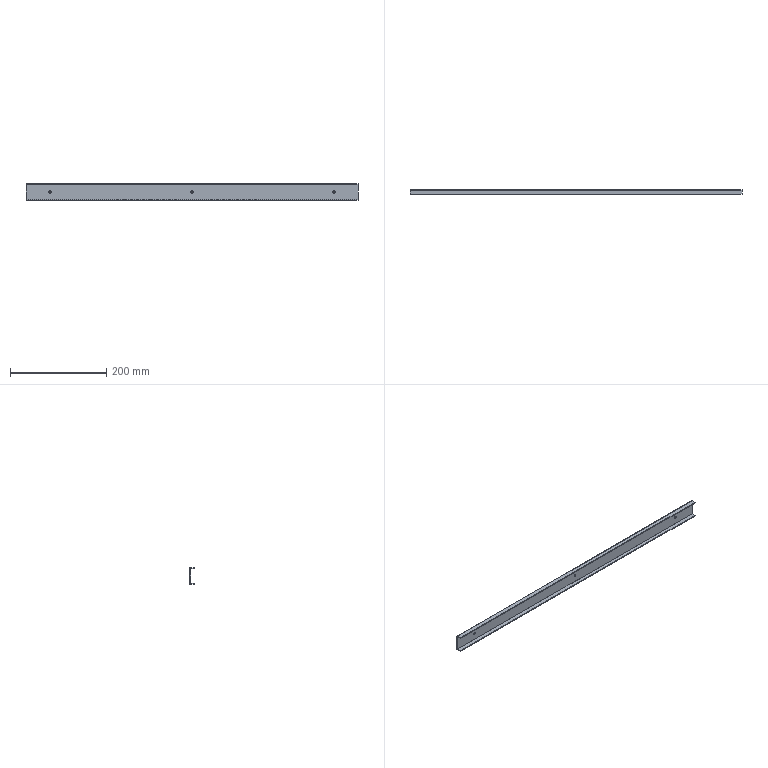Part | STEP file | Sliding Door Spacer Block | 1 solid | 20 faces | box 690 x 10 x 35 mm | volume 68950 mm3 | cylinder 10 | plane 10 | commonest cylinder face diameters 5.2 x6 0.2 x2 4.2 x2
STEP:
#1=CARTESIAN_POINT('',(-30.031,-2.,2.333));
#2=VERTEX_POINT('',#1);
#3=CARTESIAN_POINT('',(-30.031,-2.,-2.867));
#4=VERTEX_POINT('',#3);
#5=CARTESIAN_POINT('',(-30.031,-2.,-0.2666));
#6=DIRECTION('',(0.,-1.,0.));
#7=DIRECTION('',(0.,0.,1.));
#8=AXIS2_PLACEMENT_3D('',#5,#6,#7);
#9=CIRCLE('',#8,2.6);
#10=EDGE_CURVE('',#2,#4,#9,.T.);
#11=ORIENTED_EDGE('',*,*,#10,.T.);
#12=CARTESIAN_POINT('',(-30.031,0.,-2.867));
#13=VERTEX_POINT('',#12);
#14=CARTESIAN_POINT('',(-30.031,-2.,-2.867));
#15=DIRECTION('',(0.,1.,0.));
#16=VECTOR('',#15,1000.);
#17=LINE('',#14,#16);
#18=EDGE_CURVE('',#4,#13,#17,.T.);
#19=ORIENTED_EDGE('',*,*,#18,.T.);
#20=CARTESIAN_POINT('',(-30.031,0.,2.333));
#21=VERTEX_POINT('',#20);
#22=CARTESIAN_POINT('',(-30.031,0.,-0.2666));
#23=DIRECTION('',(0.,-1.,0.));
#24=DIRECTION('',(0.,0.,1.));
#25=AXIS2_PLACEMENT_3D('',#22,#23,#24);
#26=CIRCLE('',#25,2.6);
#27=EDGE_CURVE('',#21,#13,#26,.T.);
#28=ORIENTED_EDGE('',*,*,#27,.F.);
#29=CARTESIAN_POINT('',(-30.031,-2.,2.333));
#30=DIRECTION('',(0.,1.,0.));
#31=VECTOR('',#30,1000.);
#32=LINE('',#29,#31);
#33=EDGE_CURVE('',#2,#21,#32,.T.);
#34=ORIENTED_EDGE('',*,*,#33,.F.);
#35=EDGE_LOOP('',(#11,#19,#28,#34));
#36=FACE_OUTER_BOUND('',#35,.T.);
#37=CARTESIAN_POINT('',(-30.031,-2.,-0.2666));
#38=DIRECTION('',(0.,1.,0.));
#39=DIRECTION('',(0.,0.,1.));
#40=AXIS2_PLACEMENT_3D('',#37,#38,#39);
#41=CYLINDRICAL_SURFACE('',#40,2.6);
#42=ADVANCED_FACE('',(#36),#41,.F.);
#43=CARTESIAN_POINT('',(264.969,-2.,2.333));
#44=VERTEX_POINT('',#43);
#45=CARTESIAN_POINT('',(264.969,-2.,-2.867));
#46=VERTEX_POINT('',#45);
#47=CARTESIAN_POINT('',(264.969,-2.,-0.2666));
#48=DIRECTION('',(0.,-1.,0.));
#49=DIRECTION('',(0.,0.,1.));
#50=AXIS2_PLACEMENT_3D('',#47,#48,#49);
#51=CIRCLE('',#50,2.6);
#52=EDGE_CURVE('',#44,#46,#51,.T.);
#53=ORIENTED_EDGE('',*,*,#52,.T.);
#54=CARTESIAN_POINT('',(264.969,0.,-2.867));
#55=VERTEX_POINT('',#54);
#56=CARTESIAN_POINT('',(264.969,-2.,-2.867));
#57=DIRECTION('',(0.,1.,0.));
#58=VECTOR('',#57,1000.);
#59=LINE('',#56,#58);
#60=EDGE_CURVE('',#46,#55,#59,.T.);
#61=ORIENTED_EDGE('',*,*,#60,.T.);
#62=CARTESIAN_POINT('',(264.969,0.,2.333));
#63=VERTEX_POINT('',#62);
#64=CARTESIAN_POINT('',(264.969,0.,-0.2666));
#65=DIRECTION('',(0.,-1.,0.));
#66=DIRECTION('',(0.,0.,1.));
#67=AXIS2_PLACEMENT_3D('',#64,#65,#66);
#68=CIRCLE('',#67,2.6);
#69=EDGE_CURVE('',#63,#55,#68,.T.);
#70=ORIENTED_EDGE('',*,*,#69,.F.);
#71=CARTESIAN_POINT('',(264.969,-2.,2.333));
#72=DIRECTION('',(0.,1.,0.));
#73=VECTOR('',#72,1000.);
#74=LINE('',#71,#73);
#75=EDGE_CURVE('',#44,#63,#74,.T.);
#76=ORIENTED_EDGE('',*,*,#75,.F.);
#77=EDGE_LOOP('',(#53,#61,#70,#76));
#78=FACE_OUTER_BOUND('',#77,.T.);
#79=CARTESIAN_POINT('',(264.969,-2.,-0.2666));
#80=DIRECTION('',(0.,1.,0.));
#81=DIRECTION('',(0.,0.,1.));
#82=AXIS2_PLACEMENT_3D('',#79,#80,#81);
#83=CYLINDRICAL_SURFACE('',#82,2.6);
#84=ADVANCED_FACE('',(#78),#83,.F.);
#85=CARTESIAN_POINT('',(559.969,-2.,2.333));
#86=VERTEX_POINT('',#85);
#87=CARTESIAN_POINT('',(559.969,-2.,-2.867));
#88=VERTEX_POINT('',#87);
#89=CARTESIAN_POINT('',(559.969,-2.,-0.2666));
#90=DIRECTION('',(0.,-1.,0.));
#91=DIRECTION('',(0.,0.,1.));
#92=AXIS2_PLACEMENT_3D('',#89,#90,#91);
#93=CIRCLE('',#92,2.6);
#94=EDGE_CURVE('',#86,#88,#93,.T.);
#95=ORIENTED_EDGE('',*,*,#94,.T.);
#96=CARTESIAN_POINT('',(559.969,0.,-2.867));
#97=VERTEX_POINT('',#96);
#98=CARTESIAN_POINT('',(559.969,-2.,-2.867));
#99=DIRECTION('',(0.,1.,0.));
#100=VECTOR('',#99,1000.);
#101=LINE('',#98,#100);
#102=EDGE_CURVE('',#88,#97,#101,.T.);
#103=ORIENTED_EDGE('',*,*,#102,.T.);
#104=CARTESIAN_POINT('',(559.969,0.,2.333));
#105=VERTEX_POINT('',#104);
#106=CARTESIAN_POINT('',(559.969,0.,-0.2666));
#107=DIRECTION('',(0.,-1.,0.));
#108=DIRECTION('',(0.,0.,1.));
#109=AXIS2_PLACEMENT_3D('',#106,#107,#108);
#110=CIRCLE('',#109,2.6);
#111=EDGE_CURVE('',#105,#97,#110,.T.);
#112=ORIENTED_EDGE('',*,*,#111,.F.);
#113=CARTESIAN_POINT('',(559.969,-2.,2.333));
#114=DIRECTION('',(0.,1.,0.));
#115=VECTOR('',#114,1000.);
#116=LINE('',#113,#115);
#117=EDGE_CURVE('',#86,#105,#116,.T.);
#118=ORIENTED_EDGE('',*,*,#117,.F.);
#119=EDGE_LOOP('',(#95,#103,#112,#118));
#120=FACE_OUTER_BOUND('',#119,.T.);
#121=CARTESIAN_POINT('',(559.969,-2.,-0.2666));
#122=DIRECTION('',(0.,1.,0.));
#123=DIRECTION('',(0.,0.,1.));
#124=AXIS2_PLACEMENT_3D('',#121,#122,#123);
#125=CYLINDRICAL_SURFACE('',#124,2.6);
#126=ADVANCED_FACE('',(#120),#125,.F.);
#127=CARTESIAN_POINT('',(609.969,-2.,15.133));
#128=VERTEX_POINT('',#127);
#129=CARTESIAN_POINT('',(609.969,-2.,-15.667));
#130=VERTEX_POINT('',#129);
#131=CARTESIAN_POINT('',(609.969,-2.,0.));
#132=DIRECTION('',(0.,0.,-1.));
#133=VECTOR('',#132,1000.);
#134=LINE('',#131,#133);
#135=EDGE_CURVE('',#128,#130,#134,.T.);
#136=ORIENTED_EDGE('',*,*,#135,.F.);
#137=CARTESIAN_POINT('',(-80.031,-2.,15.133));
#138=VERTEX_POINT('',#137);
#139=CARTESIAN_POINT('',(0.,-2.,15.133));
#140=DIRECTION('',(1.,0.,0.));
#141=VECTOR('',#140,1000.);
#142=LINE('',#139,#141);
#143=EDGE_CURVE('',#138,#128,#142,.T.);
#144=ORIENTED_EDGE('',*,*,#143,.F.);
#145=CARTESIAN_POINT('',(-80.031,-2.,-15.667));
#146=VERTEX_POINT('',#145);
#147=CARTESIAN_POINT('',(-80.031,-2.,0.));
#148=DIRECTION('',(0.,0.,1.));
#149=VECTOR('',#148,1000.);
#150=LINE('',#147,#149);
#151=EDGE_CURVE('',#146,#138,#150,.T.);
#152=ORIENTED_EDGE('',*,*,#151,.F.);
#153=CARTESIAN_POINT('',(0.,-2.,-15.667));
#154=DIRECTION('',(-1.,0.,0.));
#155=VECTOR('',#154,1000.);
#156=LINE('',#153,#155);
#157=EDGE_CURVE('',#130,#146,#156,.T.);
#158=ORIENTED_EDGE('',*,*,#157,.F.);
#159=EDGE_LOOP('',(#136,#144,#152,#158));
#160=FACE_OUTER_BOUND('',#159,.T.);
#161=ORIENTED_EDGE('',*,*,#10,.F.);
#162=CARTESIAN_POINT('',(-30.031,-2.,-0.2666));
#163=DIRECTION('',(0.,-1.,0.));
#164=DIRECTION('',(0.,0.,1.));
#165=AXIS2_PLACEMENT_3D('',#162,#163,#164);
#166=CIRCLE('',#165,2.6);
#167=EDGE_CURVE('',#4,#2,#166,.T.);
#168=ORIENTED_EDGE('',*,*,#167,.F.);
#169=EDGE_LOOP('',(#161,#168));
#170=FACE_BOUND('',#169,.T.);
#171=ORIENTED_EDGE('',*,*,#52,.F.);
#172=CARTESIAN_POINT('',(264.969,-2.,-0.2666));
#173=DIRECTION('',(0.,-1.,0.));
#174=DIRECTION('',(0.,0.,1.));
#175=AXIS2_PLACEMENT_3D('',#172,#173,#174);
#176=CIRCLE('',#175,2.6);
#177=EDGE_CURVE('',#46,#44,#176,.T.);
#178=ORIENTED_EDGE('',*,*,#177,.F.);
#179=EDGE_LOOP('',(#171,#178));
#180=FACE_BOUND('',#179,.T.);
#181=ORIENTED_EDGE('',*,*,#94,.F.);
#182=CARTESIAN_POINT('',(559.969,-2.,-0.2666));
#183=DIRECTION('',(0.,-1.,0.));
#184=DIRECTION('',(0.,0.,1.));
#185=AXIS2_PLACEMENT_3D('',#182,#183,#184);
#186=CIRCLE('',#185,2.6);
#187=EDGE_CURVE('',#88,#86,#186,.T.);
#188=ORIENTED_EDGE('',*,*,#187,.F.);
#189=EDGE_LOOP('',(#181,#188));
#190=FACE_BOUND('',#189,.T.);
#191=CARTESIAN_POINT('',(0.,-2.,0.));
#192=DIRECTION('',(0.,1.,0.));
#193=DIRECTION('',(0.,0.,1.));
#194=AXIS2_PLACEMENT_3D('',#191,#192,#193);
#195=PLANE('',#194);
#196=ADVANCED_FACE('',(#160,#170,#180,#190),#195,.F.);
#197=CARTESIAN_POINT('',(-80.031,-2.1,-15.767));
#198=VERTEX_POINT('',#197);
#199=CARTESIAN_POINT('',(-80.031,-2.1,-15.667));
#200=DIRECTION('',(1.,0.,0.));
#201=DIRECTION('',(0.,0.,-1.));
#202=AXIS2_PLACEMENT_3D('',#199,#200,#201);
#203=CIRCLE('',#202,0.1);
#204=EDGE_CURVE('',#198,#146,#203,.T.);
#205=ORIENTED_EDGE('',*,*,#204,.F.);
#206=CARTESIAN_POINT('',(609.969,-2.1,-15.767));
#207=VERTEX_POINT('',#206);
#208=CARTESIAN_POINT('',(609.969,-2.1,-15.767));
#209=DIRECTION('',(-1.,0.,0.));
#210=VECTOR('',#209,1000.);
#211=LINE('',#208,#210);
#212=EDGE_CURVE('',#207,#198,#211,.T.);
#213=ORIENTED_EDGE('',*,*,#212,.F.);
#214=CARTESIAN_POINT('',(609.969,-2.1,-15.667));
#215=DIRECTION('',(1.,0.,0.));
#216=DIRECTION('',(0.,0.,-1.));
#217=AXIS2_PLACEMENT_3D('',#214,#215,#216);
#218=CIRCLE('',#217,0.1);
#219=EDGE_CURVE('',#207,#130,#218,.T.);
#220=ORIENTED_EDGE('',*,*,#219,.T.);
#221=ORIENTED_EDGE('',*,*,#157,.T.);
#222=EDGE_LOOP('',(#205,#213,#220,#221));
#223=FACE_OUTER_BOUND('',#222,.T.);
#224=CARTESIAN_POINT('',(609.969,-2.1,-15.667));
#225=DIRECTION('',(1.,0.,0.));
#226=DIRECTION('',(0.,0.,-1.));
#227=AXIS2_PLACEMENT_3D('',#224,#225,#226);
#228=CYLINDRICAL_SURFACE('',#227,0.1);
#229=ADVANCED_FACE('',(#223),#228,.F.);
#230=CARTESIAN_POINT('',(609.969,0.,-15.667));
#231=VERTEX_POINT('',#230);
#232=CARTESIAN_POINT('',(609.969,0.,15.133));
#233=VERTEX_POINT('',#232);
#234=CARTESIAN_POINT('',(609.969,0.,-17.767));
#235=DIRECTION('',(0.,0.,1.));
#236=VECTOR('',#235,1000.);
#237=LINE('',#234,#236);
#238=EDGE_CURVE('',#231,#233,#237,.T.);
#239=ORIENTED_EDGE('',*,*,#238,.T.);
#240=CARTESIAN_POINT('',(609.969,-2.1,17.233));
#241=VERTEX_POINT('',#240);
#242=CARTESIAN_POINT('',(609.969,-2.1,15.133));
#243=DIRECTION('',(1.,0.,0.));
#244=DIRECTION('',(0.,0.,1.));
#245=AXIS2_PLACEMENT_3D('',#242,#243,#244);
#246=CIRCLE('',#245,2.1);
#247=EDGE_CURVE('',#233,#241,#246,.T.);
#248=ORIENTED_EDGE('',*,*,#247,.T.);
#249=CARTESIAN_POINT('',(609.969,-10.,17.233));
#250=VERTEX_POINT('',#249);
#251=CARTESIAN_POINT('',(609.969,-10.,17.233));
#252=DIRECTION('',(0.,-1.,0.));
#253=VECTOR('',#252,1000.);
#254=LINE('',#251,#253);
#255=EDGE_CURVE('',#241,#250,#254,.T.);
#256=ORIENTED_EDGE('',*,*,#255,.T.);
#257=CARTESIAN_POINT('',(609.969,-10.,15.233));
#258=VERTEX_POINT('',#257);
#259=CARTESIAN_POINT('',(609.969,-10.,17.233));
#260=DIRECTION('',(0.,0.,-1.));
#261=VECTOR('',#260,1000.);
#262=LINE('',#259,#261);
#263=EDGE_CURVE('',#250,#258,#262,.T.);
#264=ORIENTED_EDGE('',*,*,#263,.T.);
#265=CARTESIAN_POINT('',(609.969,-2.1,15.233));
#266=VERTEX_POINT('',#265);
#267=CARTESIAN_POINT('',(609.969,0.,15.233));
#268=DIRECTION('',(0.,1.,0.));
#269=VECTOR('',#268,1000.);
#270=LINE('',#267,#269);
#271=EDGE_CURVE('',#258,#266,#270,.T.);
#272=ORIENTED_EDGE('',*,*,#271,.T.);
#273=CARTESIAN_POINT('',(609.969,-2.1,15.133));
#274=DIRECTION('',(-1.,0.,0.));
#275=DIRECTION('',(0.,0.,1.));
#276=AXIS2_PLACEMENT_3D('',#273,#274,#275);
#277=CIRCLE('',#276,0.1);
#278=EDGE_CURVE('',#266,#128,#277,.T.);
#279=ORIENTED_EDGE('',*,*,#278,.T.);
#280=ORIENTED_EDGE('',*,*,#135,.T.);
#281=ORIENTED_EDGE('',*,*,#219,.F.);
#282=CARTESIAN_POINT('',(609.969,-10.,-15.767));
#283=VERTEX_POINT('',#282);
#284=CARTESIAN_POINT('',(609.969,0.,-15.767));
#285=DIRECTION('',(0.,1.,0.));
#286=VECTOR('',#285,1000.);
#287=LINE('',#284,#286);
#288=EDGE_CURVE('',#283,#207,#287,.T.);
#289=ORIENTED_EDGE('',*,*,#288,.F.);
#290=CARTESIAN_POINT('',(609.969,-10.,-17.767));
#291=VERTEX_POINT('',#290);
#292=CARTESIAN_POINT('',(609.969,-10.,-17.767));
#293=DIRECTION('',(0.,0.,1.));
#294=VECTOR('',#293,1000.);
#295=LINE('',#292,#294);
#296=EDGE_CURVE('',#291,#283,#295,.T.);
#297=ORIENTED_EDGE('',*,*,#296,.F.);
#298=CARTESIAN_POINT('',(609.969,-2.1,-17.767));
#299=VERTEX_POINT('',#298);
#300=CARTESIAN_POINT('',(609.969,-10.,-17.767));
#301=DIRECTION('',(0.,1.,0.));
#302=VECTOR('',#301,1000.);
#303=LINE('',#300,#302);
#304=EDGE_CURVE('',#291,#299,#303,.T.);
#305=ORIENTED_EDGE('',*,*,#304,.T.);
#306=CARTESIAN_POINT('',(609.969,-2.1,-15.667));
#307=DIRECTION('',(-1.,0.,0.));
#308=DIRECTION('',(0.,0.,-1.));
#309=AXIS2_PLACEMENT_3D('',#306,#307,#308);
#310=CIRCLE('',#309,2.1);
#311=EDGE_CURVE('',#231,#299,#310,.T.);
#312=ORIENTED_EDGE('',*,*,#311,.F.);
#313=EDGE_LOOP('',(#239,#248,#256,#264,#272,#279,#280,#281,#289,#297,#305,#312));
#314=FACE_OUTER_BOUND('',#313,.T.);
#315=CARTESIAN_POINT('',(609.969,-2.,-17.767));
#316=DIRECTION('',(1.,0.,0.));
#317=DIRECTION('',(0.,0.,-1.));
#318=AXIS2_PLACEMENT_3D('',#315,#316,#317);
#319=PLANE('',#318);
#320=ADVANCED_FACE('',(#314),#319,.T.);
#321=ORIENTED_EDGE('',*,*,#278,.F.);
#322=CARTESIAN_POINT('',(-80.031,-2.1,15.233));
#323=VERTEX_POINT('',#322);
#324=CARTESIAN_POINT('',(-80.031,-2.1,15.233));
#325=DIRECTION('',(1.,0.,0.));
#326=VECTOR('',#325,1000.);
#327=LINE('',#324,#326);
#328=EDGE_CURVE('',#323,#266,#327,.T.);
#329=ORIENTED_EDGE('',*,*,#328,.F.);
#330=CARTESIAN_POINT('',(-80.031,-2.1,15.133));
#331=DIRECTION('',(-1.,0.,0.));
#332=DIRECTION('',(0.,0.,1.));
#333=AXIS2_PLACEMENT_3D('',#330,#331,#332);
#334=CIRCLE('',#333,0.1);
#335=EDGE_CURVE('',#323,#138,#334,.T.);
#336=ORIENTED_EDGE('',*,*,#335,.T.);
#337=ORIENTED_EDGE('',*,*,#143,.T.);
#338=EDGE_LOOP('',(#321,#329,#336,#337));
#339=FACE_OUTER_BOUND('',#338,.T.);
#340=CARTESIAN_POINT('',(-80.031,-2.1,15.133));
#341=DIRECTION('',(-1.,0.,0.));
#342=DIRECTION('',(0.,0.,1.));
#343=AXIS2_PLACEMENT_3D('',#340,#341,#342);
#344=CYLINDRICAL_SURFACE('',#343,0.1);
#345=ADVANCED_FACE('',(#339),#344,.F.);
#346=ORIENTED_EDGE('',*,*,#151,.T.);
#347=ORIENTED_EDGE('',*,*,#335,.F.);
#348=CARTESIAN_POINT('',(-80.031,-10.,15.233));
#349=VERTEX_POINT('',#348);
#350=CARTESIAN_POINT('',(-80.031,0.,15.233));
#351=DIRECTION('',(0.,-1.,0.));
#352=VECTOR('',#351,1000.);
#353=LINE('',#350,#352);
#354=EDGE_CURVE('',#323,#349,#353,.T.);
#355=ORIENTED_EDGE('',*,*,#354,.T.);
#356=CARTESIAN_POINT('',(-80.031,-10.,17.233));
#357=VERTEX_POINT('',#356);
#358=CARTESIAN_POINT('',(-80.031,-10.,17.233));
#359=DIRECTION('',(0.,0.,-1.));
#360=VECTOR('',#359,1000.);
#361=LINE('',#358,#360);
#362=EDGE_CURVE('',#357,#349,#361,.T.);
#363=ORIENTED_EDGE('',*,*,#362,.F.);
#364=CARTESIAN_POINT('',(-80.031,-2.1,17.233));
#365=VERTEX_POINT('',#364);
#366=CARTESIAN_POINT('',(-80.031,-2.,17.233));
#367=DIRECTION('',(0.,1.,0.));
#368=VECTOR('',#367,1000.);
#369=LINE('',#366,#368);
#370=EDGE_CURVE('',#357,#365,#369,.T.);
#371=ORIENTED_EDGE('',*,*,#370,.T.);
#372=CARTESIAN_POINT('',(-80.031,0.,15.133));
#373=VERTEX_POINT('',#372);
#374=CARTESIAN_POINT('',(-80.031,-2.1,15.133));
#375=DIRECTION('',(1.,0.,0.));
#376=DIRECTION('',(0.,0.,1.));
#377=AXIS2_PLACEMENT_3D('',#374,#375,#376);
#378=CIRCLE('',#377,2.1);
#379=EDGE_CURVE('',#373,#365,#378,.T.);
#380=ORIENTED_EDGE('',*,*,#379,.F.);
#381=CARTESIAN_POINT('',(-80.031,0.,-15.667));
#382=VERTEX_POINT('',#381);
#383=CARTESIAN_POINT('',(-80.031,0.,-17.767));
#384=DIRECTION('',(0.,0.,-1.));
#385=VECTOR('',#384,1000.);
#386=LINE('',#383,#385);
#387=EDGE_CURVE('',#373,#382,#386,.T.);
#388=ORIENTED_EDGE('',*,*,#387,.T.);
#389=CARTESIAN_POINT('',(-80.031,-2.1,-17.767));
#390=VERTEX_POINT('',#389);
#391=CARTESIAN_POINT('',(-80.031,-2.1,-15.667));
#392=DIRECTION('',(-1.,0.,0.));
#393=DIRECTION('',(0.,0.,-1.));
#394=AXIS2_PLACEMENT_3D('',#391,#392,#393);
#395=CIRCLE('',#394,2.1);
#396=EDGE_CURVE('',#382,#390,#395,.T.);
#397=ORIENTED_EDGE('',*,*,#396,.T.);
#398=CARTESIAN_POINT('',(-80.031,-10.,-17.767));
#399=VERTEX_POINT('',#398);
#400=CARTESIAN_POINT('',(-80.031,-2.,-17.767));
#401=DIRECTION('',(0.,-1.,0.));
#402=VECTOR('',#401,1000.);
#403=LINE('',#400,#402);
#404=EDGE_CURVE('',#390,#399,#403,.T.);
#405=ORIENTED_EDGE('',*,*,#404,.T.);
#406=CARTESIAN_POINT('',(-80.031,-10.,-15.767));
#407=VERTEX_POINT('',#406);
#408=CARTESIAN_POINT('',(-80.031,-10.,-17.767));
#409=DIRECTION('',(0.,0.,-1.));
#410=VECTOR('',#409,1000.);
#411=LINE('',#408,#410);
#412=EDGE_CURVE('',#407,#399,#411,.T.);
#413=ORIENTED_EDGE('',*,*,#412,.F.);
#414=CARTESIAN_POINT('',(-80.031,0.,-15.767));
#415=DIRECTION('',(0.,-1.,0.));
#416=VECTOR('',#415,1000.);
#417=LINE('',#414,#416);
#418=EDGE_CURVE('',#198,#407,#417,.T.);
#419=ORIENTED_EDGE('',*,*,#418,.F.);
#420=ORIENTED_EDGE('',*,*,#204,.T.);
#421=EDGE_LOOP('',(#346,#347,#355,#363,#371,#380,#388,#397,#405,#413,#419,#420));
#422=FACE_OUTER_BOUND('',#421,.T.);
#423=CARTESIAN_POINT('',(-80.031,-2.,-17.767));
#424=DIRECTION('',(-1.,0.,0.));
#425=DIRECTION('',(0.,0.,1.));
#426=AXIS2_PLACEMENT_3D('',#423,#424,#425);
#427=PLANE('',#426);
#428=ADVANCED_FACE('',(#422),#427,.T.);
#429=ORIENTED_EDGE('',*,*,#18,.F.);
#430=ORIENTED_EDGE('',*,*,#167,.T.);
#431=ORIENTED_EDGE('',*,*,#33,.T.);
#432=CARTESIAN_POINT('',(-30.031,0.,-0.2666));
#433=DIRECTION('',(0.,-1.,0.));
#434=DIRECTION('',(0.,0.,1.));
#435=AXIS2_PLACEMENT_3D('',#432,#433,#434);
#436=CIRCLE('',#435,2.6);
#437=EDGE_CURVE('',#13,#21,#436,.T.);
#438=ORIENTED_EDGE('',*,*,#437,.F.);
#439=EDGE_LOOP('',(#429,#430,#431,#438));
#440=FACE_OUTER_BOUND('',#439,.T.);
#441=CARTESIAN_POINT('',(-30.031,-2.,-0.2666));
#442=DIRECTION('',(0.,1.,0.));
#443=DIRECTION('',(0.,0.,1.));
#444=AXIS2_PLACEMENT_3D('',#441,#442,#443);
#445=CYLINDRICAL_SURFACE('',#444,2.6);
#446=ADVANCED_FACE('',(#440),#445,.F.);
#447=ORIENTED_EDGE('',*,*,#60,.F.);
#448=ORIENTED_EDGE('',*,*,#177,.T.);
#449=ORIENTED_EDGE('',*,*,#75,.T.);
#450=CARTESIAN_POINT('',(264.969,0.,-0.2666));
#451=DIRECTION('',(0.,-1.,0.));
#452=DIRECTION('',(0.,0.,1.));
#453=AXIS2_PLACEMENT_3D('',#450,#451,#452);
#454=CIRCLE('',#453,2.6);
#455=EDGE_CURVE('',#55,#63,#454,.T.);
#456=ORIENTED_EDGE('',*,*,#455,.F.);
#457=EDGE_LOOP('',(#447,#448,#449,#456));
#458=FACE_OUTER_BOUND('',#457,.T.);
#459=CARTESIAN_POINT('',(264.969,-2.,-0.2666));
#460=DIRECTION('',(0.,1.,0.));
#461=DIRECTION('',(0.,0.,1.));
#462=AXIS2_PLACEMENT_3D('',#459,#460,#461);
#463=CYLINDRICAL_SURFACE('',#462,2.6);
#464=ADVANCED_FACE('',(#458),#463,.F.);
#465=ORIENTED_EDGE('',*,*,#102,.F.);
#466=ORIENTED_EDGE('',*,*,#187,.T.);
#467=ORIENTED_EDGE('',*,*,#117,.T.);
#468=CARTESIAN_POINT('',(559.969,0.,-0.2666));
#469=DIRECTION('',(0.,-1.,0.));
#470=DIRECTION('',(0.,0.,1.));
#471=AXIS2_PLACEMENT_3D('',#468,#469,#470);
#472=CIRCLE('',#471,2.6);
#473=EDGE_CURVE('',#97,#105,#472,.T.);
#474=ORIENTED_EDGE('',*,*,#473,.F.);
#475=EDGE_LOOP('',(#465,#466,#467,#474));
#476=FACE_OUTER_BOUND('',#475,.T.);
#477=CARTESIAN_POINT('',(559.969,-2.,-0.2666));
#478=DIRECTION('',(0.,1.,0.));
#479=DIRECTION('',(0.,0.,1.));
#480=AXIS2_PLACEMENT_3D('',#477,#478,#479);
#481=CYLINDRICAL_SURFACE('',#480,2.6);
#482=ADVANCED_FACE('',(#476),#481,.F.);
#483=ORIENTED_EDGE('',*,*,#418,.T.);
#484=CARTESIAN_POINT('',(0.,-10.,-15.767));
#485=DIRECTION('',(1.,0.,0.));
#486=VECTOR('',#485,1000.);
#487=LINE('',#484,#486);
#488=EDGE_CURVE('',#407,#283,#487,.T.);
#489=ORIENTED_EDGE('',*,*,#488,.T.);
#490=ORIENTED_EDGE('',*,*,#288,.T.);
#491=ORIENTED_EDGE('',*,*,#212,.T.);
#492=EDGE_LOOP('',(#483,#489,#490,#491));
#493=FACE_OUTER_BOUND('',#492,.T.);
#494=CARTESIAN_POINT('',(0.,0.,-15.767));
#495=DIRECTION('',(0.,0.,1.));
#496=DIRECTION('',(0.,-1.,0.));
#497=AXIS2_PLACEMENT_3D('',#494,#495,#496);
#498=PLANE('',#497);
#499=ADVANCED_FACE('',(#493),#498,.T.);
#500=ORIENTED_EDGE('',*,*,#387,.F.);
#501=CARTESIAN_POINT('',(0.,0.,15.133));
#502=DIRECTION('',(1.,0.,0.));
#503=VECTOR('',#502,1000.);
#504=LINE('',#501,#503);
#505=EDGE_CURVE('',#373,#233,#504,.T.);
#506=ORIENTED_EDGE('',*,*,#505,.T.);
#507=ORIENTED_EDGE('',*,*,#238,.F.);
#508=CARTESIAN_POINT('',(0.,0.,-15.667));
#509=DIRECTION('',(-1.,0.,0.));
#510=VECTOR('',#509,1000.);
#511=LINE('',#508,#510);
#512=EDGE_CURVE('',#231,#382,#511,.T.);
#513=ORIENTED_EDGE('',*,*,#512,.T.);
#514=EDGE_LOOP('',(#500,#506,#507,#513));
#515=FACE_OUTER_BOUND('',#514,.T.);
#516=ORIENTED_EDGE('',*,*,#27,.T.);
#517=ORIENTED_EDGE('',*,*,#437,.T.);
#518=EDGE_LOOP('',(#516,#517));
#519=FACE_BOUND('',#518,.T.);
#520=ORIENTED_EDGE('',*,*,#69,.T.);
#521=ORIENTED_EDGE('',*,*,#455,.T.);
#522=EDGE_LOOP('',(#520,#521));
#523=FACE_BOUND('',#522,.T.);
#524=ORIENTED_EDGE('',*,*,#111,.T.);
#525=ORIENTED_EDGE('',*,*,#473,.T.);
#526=EDGE_LOOP('',(#524,#525));
#527=FACE_BOUND('',#526,.T.);
#528=CARTESIAN_POINT('',(0.,0.,0.));
#529=DIRECTION('',(0.,1.,0.));
#530=DIRECTION('',(0.,0.,1.));
#531=AXIS2_PLACEMENT_3D('',#528,#529,#530);
#532=PLANE('',#531);
#533=ADVANCED_FACE('',(#515,#519,#523,#527),#532,.T.);
#534=ORIENTED_EDGE('',*,*,#271,.F.);
#535=CARTESIAN_POINT('',(0.,-10.,15.233));
#536=DIRECTION('',(1.,0.,0.));
#537=VECTOR('',#536,1000.);
#538=LINE('',#535,#537);
#539=EDGE_CURVE('',#349,#258,#538,.T.);
#540=ORIENTED_EDGE('',*,*,#539,.F.);
#541=ORIENTED_EDGE('',*,*,#354,.F.);
#542=ORIENTED_EDGE('',*,*,#328,.T.);
#543=EDGE_LOOP('',(#534,#540,#541,#542));
#544=FACE_OUTER_BOUND('',#543,.T.);
#545=CARTESIAN_POINT('',(0.,0.,15.233));
#546=DIRECTION('',(0.,0.,1.));
#547=DIRECTION('',(0.,-1.,0.));
#548=AXIS2_PLACEMENT_3D('',#545,#546,#547);
#549=PLANE('',#548);
#550=ADVANCED_FACE('',(#544),#549,.F.);
#551=CARTESIAN_POINT('',(-80.031,-10.,-17.767));
#552=DIRECTION('',(1.,0.,0.));
#553=VECTOR('',#552,1000.);
#554=LINE('',#551,#553);
#555=EDGE_CURVE('',#399,#291,#554,.T.);
#556=ORIENTED_EDGE('',*,*,#555,.T.);
#557=ORIENTED_EDGE('',*,*,#296,.T.);
#558=ORIENTED_EDGE('',*,*,#488,.F.);
#559=ORIENTED_EDGE('',*,*,#412,.T.);
#560=EDGE_LOOP('',(#556,#557,#558,#559));
#561=FACE_OUTER_BOUND('',#560,.T.);
#562=CARTESIAN_POINT('',(-80.031,-10.,-17.767));
#563=DIRECTION('',(0.,-1.,0.));
#564=DIRECTION('',(0.,0.,-1.));
#565=AXIS2_PLACEMENT_3D('',#562,#563,#564);
#566=PLANE('',#565);
#567=ADVANCED_FACE('',(#561),#566,.T.);
#568=CARTESIAN_POINT('',(-80.031,-2.1,17.233));
#569=DIRECTION('',(1.,0.,0.));
#570=VECTOR('',#569,1000.);
#571=LINE('',#568,#570);
#572=EDGE_CURVE('',#365,#241,#571,.T.);
#573=ORIENTED_EDGE('',*,*,#572,.T.);
#574=ORIENTED_EDGE('',*,*,#247,.F.);
#575=ORIENTED_EDGE('',*,*,#505,.F.);
#576=ORIENTED_EDGE('',*,*,#379,.T.);
#577=EDGE_LOOP('',(#573,#574,#575,#576));
#578=FACE_OUTER_BOUND('',#577,.T.);
#579=CARTESIAN_POINT('',(-80.031,-2.1,15.133));
#580=DIRECTION('',(-1.,0.,0.));
#581=DIRECTION('',(0.,0.,1.));
#582=AXIS2_PLACEMENT_3D('',#579,#580,#581);
#583=CYLINDRICAL_SURFACE('',#582,2.1);
#584=ADVANCED_FACE('',(#578),#583,.T.);
#585=CARTESIAN_POINT('',(609.969,-2.1,-17.767));
#586=DIRECTION('',(-1.,0.,0.));
#587=VECTOR('',#586,1000.);
#588=LINE('',#585,#587);
#589=EDGE_CURVE('',#299,#390,#588,.T.);
#590=ORIENTED_EDGE('',*,*,#589,.T.);
#591=ORIENTED_EDGE('',*,*,#396,.F.);
#592=ORIENTED_EDGE('',*,*,#512,.F.);
#593=ORIENTED_EDGE('',*,*,#311,.T.);
#594=EDGE_LOOP('',(#590,#591,#592,#593));
#595=FACE_OUTER_BOUND('',#594,.T.);
#596=CARTESIAN_POINT('',(609.969,-2.1,-15.667));
#597=DIRECTION('',(1.,0.,0.));
#598=DIRECTION('',(0.,0.,-1.));
#599=AXIS2_PLACEMENT_3D('',#596,#597,#598);
#600=CYLINDRICAL_SURFACE('',#599,2.1);
#601=ADVANCED_FACE('',(#595),#600,.T.);
#602=CARTESIAN_POINT('',(-80.031,-10.,17.233));
#603=DIRECTION('',(-1.,0.,0.));
#604=VECTOR('',#603,1000.);
#605=LINE('',#602,#604);
#606=EDGE_CURVE('',#250,#357,#605,.T.);
#607=ORIENTED_EDGE('',*,*,#606,.T.);
#608=ORIENTED_EDGE('',*,*,#362,.T.);
#609=ORIENTED_EDGE('',*,*,#539,.T.);
#610=ORIENTED_EDGE('',*,*,#263,.F.);
#611=EDGE_LOOP('',(#607,#608,#609,#610));
#612=FACE_OUTER_BOUND('',#611,.T.);
#613=CARTESIAN_POINT('',(-80.031,-10.,17.233));
#614=DIRECTION('',(0.,-1.,0.));
#615=DIRECTION('',(0.,0.,-1.));
#616=AXIS2_PLACEMENT_3D('',#613,#614,#615);
#617=PLANE('',#616);
#618=ADVANCED_FACE('',(#612),#617,.T.);
#619=ORIENTED_EDGE('',*,*,#304,.F.);
#620=ORIENTED_EDGE('',*,*,#555,.F.);
#621=ORIENTED_EDGE('',*,*,#404,.F.);
#622=ORIENTED_EDGE('',*,*,#589,.F.);
#623=EDGE_LOOP('',(#619,#620,#621,#622));
#624=FACE_OUTER_BOUND('',#623,.T.);
#625=CARTESIAN_POINT('',(0.,0.,-17.767));
#626=DIRECTION('',(0.,0.,1.));
#627=DIRECTION('',(0.,-1.,0.));
#628=AXIS2_PLACEMENT_3D('',#625,#626,#627);
#629=PLANE('',#628);
#630=ADVANCED_FACE('',(#624),#629,.F.);
#631=ORIENTED_EDGE('',*,*,#370,.F.);
#632=ORIENTED_EDGE('',*,*,#606,.F.);
#633=ORIENTED_EDGE('',*,*,#255,.F.);
#634=ORIENTED_EDGE('',*,*,#572,.F.);
#635=EDGE_LOOP('',(#631,#632,#633,#634));
#636=FACE_OUTER_BOUND('',#635,.T.);
#637=CARTESIAN_POINT('',(0.,0.,17.233));
#638=DIRECTION('',(0.,0.,1.));
#639=DIRECTION('',(0.,-1.,0.));
#640=AXIS2_PLACEMENT_3D('',#637,#638,#639);
#641=PLANE('',#640);
#642=ADVANCED_FACE('',(#636),#641,.T.);
#643=CLOSED_SHELL('',(#42,#84,#126,#196,#229,#320,#345,#428,#446,#464,#482,#499,#533,#550,#567,#584,#601,#618,#630,#642));
#644=MANIFOLD_SOLID_BREP('',#643);
#645=CARTESIAN_POINT('',(0.,0.,0.));
#646=DIRECTION('',(0.,0.,1.));
#647=DIRECTION('',(1.,0.,0.));
#648=AXIS2_PLACEMENT_3D('',#645,#646,#647);
#649=(LENGTH_UNIT()NAMED_UNIT(*)SI_UNIT(.MILLI.,.METRE.));
#650=UNCERTAINTY_MEASURE_WITH_UNIT(LENGTH_MEASURE(0.00001),#649,'','');
#651=(NAMED_UNIT(*)PLANE_ANGLE_UNIT()SI_UNIT($,.RADIAN.));
#652=(NAMED_UNIT(*)SI_UNIT($,.STERADIAN.)SOLID_ANGLE_UNIT());
#653=(GEOMETRIC_REPRESENTATION_CONTEXT(3)GLOBAL_UNCERTAINTY_ASSIGNED_CONTEXT((#650))GLOBAL_UNIT_ASSIGNED_CONTEXT((#649,#651,#652))REPRESENTATION_CONTEXT('',''));
#654=ADVANCED_BREP_SHAPE_REPRESENTATION('',(#644,#648),#653);